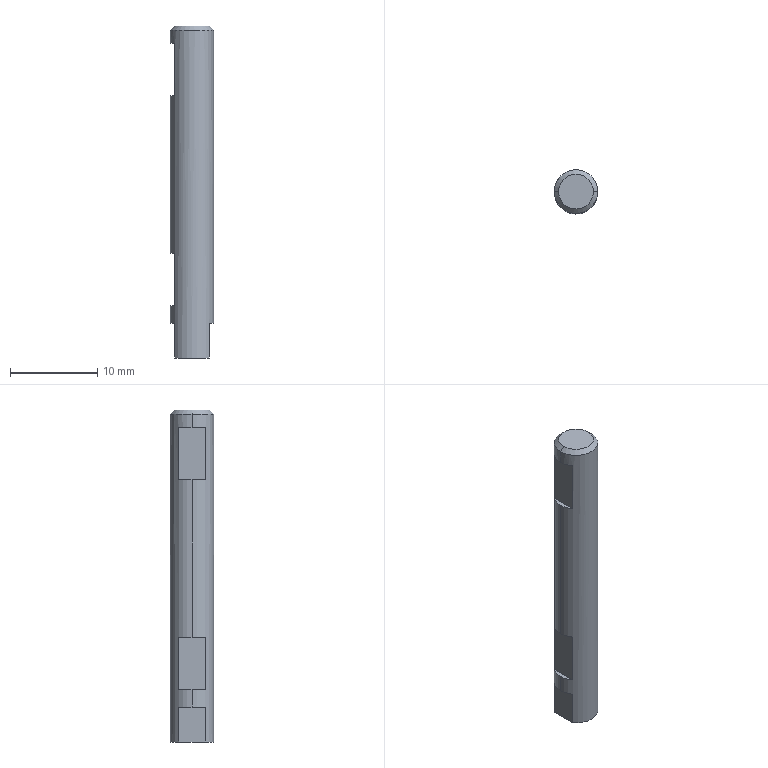Part | STEP file | PN_0012 Mount electronic clip wheel shaft A | 1 solid | 16 faces | box 5 x 5 x 38 mm | volume 723.858 mm3 | plane 12 | cone 2 | cylinder 2 | commonest cylinder face diameters 5 x2
STEP:
#1=CARTESIAN_POINT('',(0.,0.,0.));
#2=DIRECTION('',(0.,0.,1.));
#3=DIRECTION('',(1.,0.,0.));
#4=AXIS2_PLACEMENT_3D('',#1,#2,#3);
#5=CARTESIAN_POINT('',(2.,0.,38.));
#6=VERTEX_POINT('',#5);
#7=CARTESIAN_POINT('',(-2.,0.,38.));
#8=VERTEX_POINT('',#7);
#9=CARTESIAN_POINT('',(0.,0.,38.));
#10=DIRECTION('',(0.,0.,1.));
#11=DIRECTION('',(1.,0.,0.));
#12=AXIS2_PLACEMENT_3D('',#9,#10,#11);
#13=CIRCLE('',#12,2.);
#14=CARTESIAN_POINT('',(0.,0.,38.));
#15=DIRECTION('',(0.,0.,-1.));
#16=DIRECTION('',(-1.,0.,0.));
#17=AXIS2_PLACEMENT_3D('',#14,#15,#16);
#18=CONICAL_SURFACE('',#17,2.,0.7854);
#19=CARTESIAN_POINT('',(3.142,0.));
#20=DIRECTION('',(-1.,0.));
#21=VECTOR('',#20,1.);
#22=LINE('',#19,#21);
#23=(GEOMETRIC_REPRESENTATION_CONTEXT(2)PARAMETRIC_REPRESENTATION_CONTEXT()REPRESENTATION_CONTEXT('',''));
#24=DEFINITIONAL_REPRESENTATION('',(#22),#23);
#25=PCURVE('',#18,#24);
#26=CARTESIAN_POINT('',(0.,0.,38.));
#27=DIRECTION('',(0.,0.,1.));
#28=DIRECTION('',(1.,0.,0.));
#29=AXIS2_PLACEMENT_3D('',#26,#27,#28);
#30=PLANE('',#29);
#31=CARTESIAN_POINT('',(0.,0.));
#32=DIRECTION('',(1.,0.));
#33=AXIS2_PLACEMENT_2D('',#31,#32);
#34=CIRCLE('',#33,2.);
#35=(GEOMETRIC_REPRESENTATION_CONTEXT(2)PARAMETRIC_REPRESENTATION_CONTEXT()REPRESENTATION_CONTEXT('',''));
#36=DEFINITIONAL_REPRESENTATION('',(#34),#35);
#37=PCURVE('',#30,#36);
#38=SURFACE_CURVE('',#13,(#25,#37),.PCURVE_S1.);
#39=EDGE_CURVE('',#6,#8,#38,.T.);
#40=ORIENTED_EDGE('',*,*,#39,.F.);
#41=CARTESIAN_POINT('',(2.5,0.,37.5));
#42=VERTEX_POINT('',#41);
#43=CARTESIAN_POINT('',(2.,0.,38.));
#44=DIRECTION('',(0.7071,0.,-0.7071));
#45=VECTOR('',#44,1.);
#46=LINE('',#43,#45);
#47=CARTESIAN_POINT('',(3.142,0.));
#48=DIRECTION('',(0.,1.));
#49=VECTOR('',#48,1.);
#50=LINE('',#47,#49);
#51=(GEOMETRIC_REPRESENTATION_CONTEXT(2)PARAMETRIC_REPRESENTATION_CONTEXT()REPRESENTATION_CONTEXT('',''));
#52=DEFINITIONAL_REPRESENTATION('',(#50),#51);
#53=PCURVE('',#18,#52);
#54=CARTESIAN_POINT('',(0.,0.,38.));
#55=DIRECTION('',(0.,0.,-1.));
#56=DIRECTION('',(-1.,0.,0.));
#57=AXIS2_PLACEMENT_3D('',#54,#55,#56);
#58=CONICAL_SURFACE('',#57,2.,0.7854);
#59=CARTESIAN_POINT('',(3.142,0.));
#60=DIRECTION('',(0.,1.));
#61=VECTOR('',#60,1.);
#62=LINE('',#59,#61);
#63=(GEOMETRIC_REPRESENTATION_CONTEXT(2)PARAMETRIC_REPRESENTATION_CONTEXT()REPRESENTATION_CONTEXT('',''));
#64=DEFINITIONAL_REPRESENTATION('',(#62),#63);
#65=PCURVE('',#58,#64);
#66=SURFACE_CURVE('',#46,(#53,#65),.PCURVE_S1.);
#67=EDGE_CURVE('',#6,#42,#66,.T.);
#68=ORIENTED_EDGE('',*,*,#67,.T.);
#69=CARTESIAN_POINT('',(-2.5,0.,37.5));
#70=VERTEX_POINT('',#69);
#71=CARTESIAN_POINT('',(0.,0.,37.5));
#72=DIRECTION('',(0.,0.,-1.));
#73=DIRECTION('',(1.,0.,0.));
#74=AXIS2_PLACEMENT_3D('',#71,#72,#73);
#75=CIRCLE('',#74,2.5);
#76=CARTESIAN_POINT('',(-3.142,0.5));
#77=DIRECTION('',(1.,0.));
#78=VECTOR('',#77,1.);
#79=LINE('',#76,#78);
#80=(GEOMETRIC_REPRESENTATION_CONTEXT(2)PARAMETRIC_REPRESENTATION_CONTEXT()REPRESENTATION_CONTEXT('',''));
#81=DEFINITIONAL_REPRESENTATION('',(#79),#80);
#82=PCURVE('',#18,#81);
#83=CARTESIAN_POINT('',(0.,0.,38.));
#84=DIRECTION('',(0.,0.,-1.));
#85=DIRECTION('',(-1.,0.,0.));
#86=AXIS2_PLACEMENT_3D('',#83,#84,#85);
#87=CYLINDRICAL_SURFACE('',#86,2.5);
#88=CARTESIAN_POINT('',(-3.142,0.5));
#89=DIRECTION('',(1.,0.));
#90=VECTOR('',#89,1.);
#91=LINE('',#88,#90);
#92=(GEOMETRIC_REPRESENTATION_CONTEXT(2)PARAMETRIC_REPRESENTATION_CONTEXT()REPRESENTATION_CONTEXT('',''));
#93=DEFINITIONAL_REPRESENTATION('',(#91),#92);
#94=PCURVE('',#87,#93);
#95=SURFACE_CURVE('',#75,(#82,#94),.PCURVE_S1.);
#96=EDGE_CURVE('',#70,#42,#95,.T.);
#97=ORIENTED_EDGE('',*,*,#96,.F.);
#98=CARTESIAN_POINT('',(-2.,0.,38.));
#99=DIRECTION('',(-0.7071,0.,-0.7071));
#100=VECTOR('',#99,1.);
#101=LINE('',#98,#100);
#102=CARTESIAN_POINT('',(0.,0.));
#103=DIRECTION('',(0.,1.));
#104=VECTOR('',#103,1.);
#105=LINE('',#102,#104);
#106=(GEOMETRIC_REPRESENTATION_CONTEXT(2)PARAMETRIC_REPRESENTATION_CONTEXT()REPRESENTATION_CONTEXT('',''));
#107=DEFINITIONAL_REPRESENTATION('',(#105),#106);
#108=PCURVE('',#18,#107);
#109=CARTESIAN_POINT('',(6.283,0.));
#110=DIRECTION('',(0.,1.));
#111=VECTOR('',#110,1.);
#112=LINE('',#109,#111);
#113=(GEOMETRIC_REPRESENTATION_CONTEXT(2)PARAMETRIC_REPRESENTATION_CONTEXT()REPRESENTATION_CONTEXT('',''));
#114=DEFINITIONAL_REPRESENTATION('',(#112),#113);
#115=PCURVE('',#58,#114);
#116=SURFACE_CURVE('',#101,(#108,#115),.PCURVE_S1.);
#117=EDGE_CURVE('',#8,#70,#116,.T.);
#118=ORIENTED_EDGE('',*,*,#117,.F.);
#119=EDGE_LOOP('',(#40,#68,#97,#118));
#120=FACE_BOUND('',#119,.T.);
#121=ADVANCED_FACE('',(#120),#18,.T.);
#122=ORIENTED_EDGE('',*,*,#96,.T.);
#123=CARTESIAN_POINT('',(2.5,0.,4.));
#124=VERTEX_POINT('',#123);
#125=CARTESIAN_POINT('',(2.5,0.,38.));
#126=DIRECTION('',(0.,0.,-1.));
#127=VECTOR('',#126,1.);
#128=LINE('',#125,#127);
#129=CARTESIAN_POINT('',(3.142,0.));
#130=DIRECTION('',(0.,1.));
#131=VECTOR('',#130,1.);
#132=LINE('',#129,#131);
#133=(GEOMETRIC_REPRESENTATION_CONTEXT(2)PARAMETRIC_REPRESENTATION_CONTEXT()REPRESENTATION_CONTEXT('',''));
#134=DEFINITIONAL_REPRESENTATION('',(#132),#133);
#135=PCURVE('',#87,#134);
#136=CARTESIAN_POINT('',(0.,0.,38.));
#137=DIRECTION('',(0.,0.,-1.));
#138=DIRECTION('',(-1.,0.,0.));
#139=AXIS2_PLACEMENT_3D('',#136,#137,#138);
#140=CYLINDRICAL_SURFACE('',#139,2.5);
#141=CARTESIAN_POINT('',(3.142,0.));
#142=DIRECTION('',(0.,1.));
#143=VECTOR('',#142,1.);
#144=LINE('',#141,#143);
#145=(GEOMETRIC_REPRESENTATION_CONTEXT(2)PARAMETRIC_REPRESENTATION_CONTEXT()REPRESENTATION_CONTEXT('',''));
#146=DEFINITIONAL_REPRESENTATION('',(#144),#145);
#147=PCURVE('',#140,#146);
#148=SURFACE_CURVE('',#128,(#135,#147),.PCURVE_S1.);
#149=EDGE_CURVE('',#42,#124,#148,.T.);
#150=ORIENTED_EDGE('',*,*,#149,.T.);
#151=CARTESIAN_POINT('',(2.,1.5,4.));
#152=VERTEX_POINT('',#151);
#153=CARTESIAN_POINT('',(0.,0.,4.));
#154=DIRECTION('',(0.,0.,-1.));
#155=DIRECTION('',(-1.,0.,0.));
#156=AXIS2_PLACEMENT_3D('',#153,#154,#155);
#157=CIRCLE('',#156,2.5);
#158=CARTESIAN_POINT('',(0.,34.));
#159=DIRECTION('',(1.,0.));
#160=VECTOR('',#159,1.);
#161=LINE('',#158,#160);
#162=(GEOMETRIC_REPRESENTATION_CONTEXT(2)PARAMETRIC_REPRESENTATION_CONTEXT()REPRESENTATION_CONTEXT('',''));
#163=DEFINITIONAL_REPRESENTATION('',(#161),#162);
#164=PCURVE('',#87,#163);
#165=CARTESIAN_POINT('',(0.,0.,4.));
#166=DIRECTION('',(0.,0.,-1.));
#167=DIRECTION('',(-1.,0.,0.));
#168=AXIS2_PLACEMENT_3D('',#165,#166,#167);
#169=PLANE('',#168);
#170=CARTESIAN_POINT('',(0.,0.));
#171=DIRECTION('',(1.,0.));
#172=AXIS2_PLACEMENT_2D('',#170,#171);
#173=CIRCLE('',#172,2.5);
#174=(GEOMETRIC_REPRESENTATION_CONTEXT(2)PARAMETRIC_REPRESENTATION_CONTEXT()REPRESENTATION_CONTEXT('',''));
#175=DEFINITIONAL_REPRESENTATION('',(#173),#174);
#176=PCURVE('',#169,#175);
#177=SURFACE_CURVE('',#157,(#164,#176),.PCURVE_S1.);
#178=EDGE_CURVE('',#152,#124,#177,.T.);
#179=ORIENTED_EDGE('',*,*,#178,.F.);
#180=CARTESIAN_POINT('',(2.,1.5,0.));
#181=VERTEX_POINT('',#180);
#182=CARTESIAN_POINT('',(2.,1.5,38.));
#183=DIRECTION('',(0.,0.,-1.));
#184=VECTOR('',#183,1.);
#185=LINE('',#182,#184);
#186=CARTESIAN_POINT('',(2.498,0.));
#187=DIRECTION('',(0.,1.));
#188=VECTOR('',#187,1.);
#189=LINE('',#186,#188);
#190=(GEOMETRIC_REPRESENTATION_CONTEXT(2)PARAMETRIC_REPRESENTATION_CONTEXT()REPRESENTATION_CONTEXT('',''));
#191=DEFINITIONAL_REPRESENTATION('',(#189),#190);
#192=PCURVE('',#87,#191);
#193=CARTESIAN_POINT('',(2.,0.,4.));
#194=DIRECTION('',(-1.,0.,0.));
#195=DIRECTION('',(0.,0.,1.));
#196=AXIS2_PLACEMENT_3D('',#193,#194,#195);
#197=PLANE('',#196);
#198=CARTESIAN_POINT('',(34.,1.5));
#199=DIRECTION('',(-1.,0.));
#200=VECTOR('',#199,1.);
#201=LINE('',#198,#200);
#202=(GEOMETRIC_REPRESENTATION_CONTEXT(2)PARAMETRIC_REPRESENTATION_CONTEXT()REPRESENTATION_CONTEXT('',''));
#203=DEFINITIONAL_REPRESENTATION('',(#201),#202);
#204=PCURVE('',#197,#203);
#205=SURFACE_CURVE('',#185,(#192,#204),.PCURVE_S1.);
#206=EDGE_CURVE('',#152,#181,#205,.T.);
#207=ORIENTED_EDGE('',*,*,#206,.T.);
#208=CARTESIAN_POINT('',(-2.,1.5,0.));
#209=VERTEX_POINT('',#208);
#210=CARTESIAN_POINT('',(0.,0.,0.));
#211=DIRECTION('',(0.,0.,1.));
#212=DIRECTION('',(1.,0.,0.));
#213=AXIS2_PLACEMENT_3D('',#210,#211,#212);
#214=CIRCLE('',#213,2.5);
#215=CARTESIAN_POINT('',(3.142,38.));
#216=DIRECTION('',(-1.,0.));
#217=VECTOR('',#216,1.);
#218=LINE('',#215,#217);
#219=(GEOMETRIC_REPRESENTATION_CONTEXT(2)PARAMETRIC_REPRESENTATION_CONTEXT()REPRESENTATION_CONTEXT('',''));
#220=DEFINITIONAL_REPRESENTATION('',(#218),#219);
#221=PCURVE('',#87,#220);
#222=CARTESIAN_POINT('',(0.,0.,0.));
#223=DIRECTION('',(0.,0.,1.));
#224=DIRECTION('',(1.,0.,0.));
#225=AXIS2_PLACEMENT_3D('',#222,#223,#224);
#226=PLANE('',#225);
#227=CARTESIAN_POINT('',(0.,0.));
#228=DIRECTION('',(1.,0.));
#229=AXIS2_PLACEMENT_2D('',#227,#228);
#230=CIRCLE('',#229,2.5);
#231=(GEOMETRIC_REPRESENTATION_CONTEXT(2)PARAMETRIC_REPRESENTATION_CONTEXT()REPRESENTATION_CONTEXT('',''));
#232=DEFINITIONAL_REPRESENTATION('',(#230),#231);
#233=PCURVE('',#226,#232);
#234=SURFACE_CURVE('',#214,(#221,#233),.PCURVE_S1.);
#235=EDGE_CURVE('',#181,#209,#234,.T.);
#236=ORIENTED_EDGE('',*,*,#235,.T.);
#237=CARTESIAN_POINT('',(-2.,1.5,4.));
#238=VERTEX_POINT('',#237);
#239=CARTESIAN_POINT('',(-2.,1.5,38.));
#240=DIRECTION('',(0.,0.,-1.));
#241=VECTOR('',#240,1.);
#242=LINE('',#239,#241);
#243=CARTESIAN_POINT('',(0.6435,0.));
#244=DIRECTION('',(0.,1.));
#245=VECTOR('',#244,1.);
#246=LINE('',#243,#245);
#247=(GEOMETRIC_REPRESENTATION_CONTEXT(2)PARAMETRIC_REPRESENTATION_CONTEXT()REPRESENTATION_CONTEXT('',''));
#248=DEFINITIONAL_REPRESENTATION('',(#246),#247);
#249=PCURVE('',#87,#248);
#250=CARTESIAN_POINT('',(-2.,0.,4.));
#251=DIRECTION('',(-1.,0.,0.));
#252=DIRECTION('',(0.,0.,1.));
#253=AXIS2_PLACEMENT_3D('',#250,#251,#252);
#254=PLANE('',#253);
#255=CARTESIAN_POINT('',(34.,1.5));
#256=DIRECTION('',(-1.,0.));
#257=VECTOR('',#256,1.);
#258=LINE('',#255,#257);
#259=(GEOMETRIC_REPRESENTATION_CONTEXT(2)PARAMETRIC_REPRESENTATION_CONTEXT()REPRESENTATION_CONTEXT('',''));
#260=DEFINITIONAL_REPRESENTATION('',(#258),#259);
#261=PCURVE('',#254,#260);
#262=SURFACE_CURVE('',#242,(#249,#261),.PCURVE_S1.);
#263=EDGE_CURVE('',#238,#209,#262,.T.);
#264=ORIENTED_EDGE('',*,*,#263,.F.);
#265=CARTESIAN_POINT('',(-2.5,0.,4.));
#266=VERTEX_POINT('',#265);
#267=CARTESIAN_POINT('',(0.,0.,4.));
#268=DIRECTION('',(0.,0.,-1.));
#269=DIRECTION('',(-1.,0.,0.));
#270=AXIS2_PLACEMENT_3D('',#267,#268,#269);
#271=CIRCLE('',#270,2.5);
#272=CARTESIAN_POINT('',(0.,34.));
#273=DIRECTION('',(1.,0.));
#274=VECTOR('',#273,1.);
#275=LINE('',#272,#274);
#276=(GEOMETRIC_REPRESENTATION_CONTEXT(2)PARAMETRIC_REPRESENTATION_CONTEXT()REPRESENTATION_CONTEXT('',''));
#277=DEFINITIONAL_REPRESENTATION('',(#275),#276);
#278=PCURVE('',#87,#277);
#279=CARTESIAN_POINT('',(0.,0.,4.));
#280=DIRECTION('',(0.,0.,-1.));
#281=DIRECTION('',(-1.,0.,0.));
#282=AXIS2_PLACEMENT_3D('',#279,#280,#281);
#283=PLANE('',#282);
#284=CARTESIAN_POINT('',(0.,0.));
#285=DIRECTION('',(1.,0.));
#286=AXIS2_PLACEMENT_2D('',#284,#285);
#287=CIRCLE('',#286,2.5);
#288=(GEOMETRIC_REPRESENTATION_CONTEXT(2)PARAMETRIC_REPRESENTATION_CONTEXT()REPRESENTATION_CONTEXT('',''));
#289=DEFINITIONAL_REPRESENTATION('',(#287),#288);
#290=PCURVE('',#283,#289);
#291=SURFACE_CURVE('',#271,(#278,#290),.PCURVE_S1.);
#292=EDGE_CURVE('',#266,#238,#291,.T.);
#293=ORIENTED_EDGE('',*,*,#292,.F.);
#294=CARTESIAN_POINT('',(-2.5,0.,6.));
#295=VERTEX_POINT('',#294);
#296=CARTESIAN_POINT('',(-2.5,0.,38.));
#297=DIRECTION('',(0.,0.,-1.));
#298=VECTOR('',#297,1.);
#299=LINE('',#296,#298);
#300=CARTESIAN_POINT('',(0.,0.));
#301=DIRECTION('',(0.,1.));
#302=VECTOR('',#301,1.);
#303=LINE('',#300,#302);
#304=(GEOMETRIC_REPRESENTATION_CONTEXT(2)PARAMETRIC_REPRESENTATION_CONTEXT()REPRESENTATION_CONTEXT('',''));
#305=DEFINITIONAL_REPRESENTATION('',(#303),#304);
#306=PCURVE('',#87,#305);
#307=CARTESIAN_POINT('',(6.283,0.));
#308=DIRECTION('',(0.,1.));
#309=VECTOR('',#308,1.);
#310=LINE('',#307,#309);
#311=(GEOMETRIC_REPRESENTATION_CONTEXT(2)PARAMETRIC_REPRESENTATION_CONTEXT()REPRESENTATION_CONTEXT('',''));
#312=DEFINITIONAL_REPRESENTATION('',(#310),#311);
#313=PCURVE('',#140,#312);
#314=SURFACE_CURVE('',#299,(#306,#313),.PCURVE_S1.);
#315=EDGE_CURVE('',#295,#266,#314,.T.);
#316=ORIENTED_EDGE('',*,*,#315,.F.);
#317=CARTESIAN_POINT('',(-2.,1.5,6.));
#318=VERTEX_POINT('',#317);
#319=CARTESIAN_POINT('',(0.,0.,6.));
#320=DIRECTION('',(0.,0.,1.));
#321=DIRECTION('',(1.,0.,0.));
#322=AXIS2_PLACEMENT_3D('',#319,#320,#321);
#323=CIRCLE('',#322,2.5);
#324=CARTESIAN_POINT('',(3.142,32.));
#325=DIRECTION('',(-1.,0.));
#326=VECTOR('',#325,1.);
#327=LINE('',#324,#326);
#328=(GEOMETRIC_REPRESENTATION_CONTEXT(2)PARAMETRIC_REPRESENTATION_CONTEXT()REPRESENTATION_CONTEXT('',''));
#329=DEFINITIONAL_REPRESENTATION('',(#327),#328);
#330=PCURVE('',#87,#329);
#331=CARTESIAN_POINT('',(-5.963,40.,6.));
#332=DIRECTION('',(0.,0.,1.));
#333=DIRECTION('',(1.,0.,0.));
#334=AXIS2_PLACEMENT_3D('',#331,#332,#333);
#335=PLANE('',#334);
#336=CARTESIAN_POINT('',(5.963,-40.));
#337=DIRECTION('',(1.,0.));
#338=AXIS2_PLACEMENT_2D('',#336,#337);
#339=CIRCLE('',#338,2.5);
#340=(GEOMETRIC_REPRESENTATION_CONTEXT(2)PARAMETRIC_REPRESENTATION_CONTEXT()REPRESENTATION_CONTEXT('',''));
#341=DEFINITIONAL_REPRESENTATION('',(#339),#340);
#342=PCURVE('',#335,#341);
#343=SURFACE_CURVE('',#323,(#330,#342),.PCURVE_S1.);
#344=EDGE_CURVE('',#318,#295,#343,.T.);
#345=ORIENTED_EDGE('',*,*,#344,.F.);
#346=CARTESIAN_POINT('',(-2.,1.5,12.));
#347=VERTEX_POINT('',#346);
#348=CARTESIAN_POINT('',(-2.,1.5,38.));
#349=DIRECTION('',(0.,0.,-1.));
#350=VECTOR('',#349,1.);
#351=LINE('',#348,#350);
#352=CARTESIAN_POINT('',(0.6435,0.));
#353=DIRECTION('',(0.,1.));
#354=VECTOR('',#353,1.);
#355=LINE('',#352,#354);
#356=(GEOMETRIC_REPRESENTATION_CONTEXT(2)PARAMETRIC_REPRESENTATION_CONTEXT()REPRESENTATION_CONTEXT('',''));
#357=DEFINITIONAL_REPRESENTATION('',(#355),#356);
#358=PCURVE('',#87,#357);
#359=CARTESIAN_POINT('',(-2.,40.,6.));
#360=DIRECTION('',(-1.,0.,0.));
#361=DIRECTION('',(0.,0.,1.));
#362=AXIS2_PLACEMENT_3D('',#359,#360,#361);
#363=PLANE('',#362);
#364=CARTESIAN_POINT('',(32.,-38.5));
#365=DIRECTION('',(-1.,0.));
#366=VECTOR('',#365,1.);
#367=LINE('',#364,#366);
#368=(GEOMETRIC_REPRESENTATION_CONTEXT(2)PARAMETRIC_REPRESENTATION_CONTEXT()REPRESENTATION_CONTEXT('',''));
#369=DEFINITIONAL_REPRESENTATION('',(#367),#368);
#370=PCURVE('',#363,#369);
#371=SURFACE_CURVE('',#351,(#358,#370),.PCURVE_S1.);
#372=EDGE_CURVE('',#347,#318,#371,.T.);
#373=ORIENTED_EDGE('',*,*,#372,.F.);
#374=CARTESIAN_POINT('',(-2.5,0.,12.));
#375=VERTEX_POINT('',#374);
#376=CARTESIAN_POINT('',(0.,0.,12.));
#377=DIRECTION('',(0.,0.,-1.));
#378=DIRECTION('',(-1.,0.,0.));
#379=AXIS2_PLACEMENT_3D('',#376,#377,#378);
#380=CIRCLE('',#379,2.5);
#381=CARTESIAN_POINT('',(0.,26.));
#382=DIRECTION('',(1.,0.));
#383=VECTOR('',#382,1.);
#384=LINE('',#381,#383);
#385=(GEOMETRIC_REPRESENTATION_CONTEXT(2)PARAMETRIC_REPRESENTATION_CONTEXT()REPRESENTATION_CONTEXT('',''));
#386=DEFINITIONAL_REPRESENTATION('',(#384),#385);
#387=PCURVE('',#87,#386);
#388=CARTESIAN_POINT('',(-5.963,40.,12.));
#389=DIRECTION('',(0.,0.,-1.));
#390=DIRECTION('',(-1.,0.,0.));
#391=AXIS2_PLACEMENT_3D('',#388,#389,#390);
#392=PLANE('',#391);
#393=CARTESIAN_POINT('',(-5.963,-40.));
#394=DIRECTION('',(1.,0.));
#395=AXIS2_PLACEMENT_2D('',#393,#394);
#396=CIRCLE('',#395,2.5);
#397=(GEOMETRIC_REPRESENTATION_CONTEXT(2)PARAMETRIC_REPRESENTATION_CONTEXT()REPRESENTATION_CONTEXT('',''));
#398=DEFINITIONAL_REPRESENTATION('',(#396),#397);
#399=PCURVE('',#392,#398);
#400=SURFACE_CURVE('',#380,(#387,#399),.PCURVE_S1.);
#401=EDGE_CURVE('',#375,#347,#400,.T.);
#402=ORIENTED_EDGE('',*,*,#401,.F.);
#403=CARTESIAN_POINT('',(-2.5,0.,30.));
#404=VERTEX_POINT('',#403);
#405=CARTESIAN_POINT('',(-2.5,0.,38.));
#406=DIRECTION('',(0.,0.,-1.));
#407=VECTOR('',#406,1.);
#408=LINE('',#405,#407);
#409=CARTESIAN_POINT('',(0.,0.));
#410=DIRECTION('',(0.,1.));
#411=VECTOR('',#410,1.);
#412=LINE('',#409,#411);
#413=(GEOMETRIC_REPRESENTATION_CONTEXT(2)PARAMETRIC_REPRESENTATION_CONTEXT()REPRESENTATION_CONTEXT('',''));
#414=DEFINITIONAL_REPRESENTATION('',(#412),#413);
#415=PCURVE('',#87,#414);
#416=CARTESIAN_POINT('',(6.283,0.));
#417=DIRECTION('',(0.,1.));
#418=VECTOR('',#417,1.);
#419=LINE('',#416,#418);
#420=(GEOMETRIC_REPRESENTATION_CONTEXT(2)PARAMETRIC_REPRESENTATION_CONTEXT()REPRESENTATION_CONTEXT('',''));
#421=DEFINITIONAL_REPRESENTATION('',(#419),#420);
#422=PCURVE('',#140,#421);
#423=SURFACE_CURVE('',#408,(#415,#422),.PCURVE_S1.);
#424=EDGE_CURVE('',#404,#375,#423,.T.);
#425=ORIENTED_EDGE('',*,*,#424,.F.);
#426=CARTESIAN_POINT('',(-2.,1.5,30.));
#427=VERTEX_POINT('',#426);
#428=CARTESIAN_POINT('',(0.,0.,30.));
#429=DIRECTION('',(0.,0.,1.));
#430=DIRECTION('',(1.,0.,0.));
#431=AXIS2_PLACEMENT_3D('',#428,#429,#430);
#432=CIRCLE('',#431,2.5);
#433=CARTESIAN_POINT('',(3.142,8.));
#434=DIRECTION('',(-1.,0.));
#435=VECTOR('',#434,1.);
#436=LINE('',#433,#435);
#437=(GEOMETRIC_REPRESENTATION_CONTEXT(2)PARAMETRIC_REPRESENTATION_CONTEXT()REPRESENTATION_CONTEXT('',''));
#438=DEFINITIONAL_REPRESENTATION('',(#436),#437);
#439=PCURVE('',#87,#438);
#440=CARTESIAN_POINT('',(-4.8,40.,30.));
#441=DIRECTION('',(0.,0.,1.));
#442=DIRECTION('',(1.,0.,0.));
#443=AXIS2_PLACEMENT_3D('',#440,#441,#442);
#444=PLANE('',#443);
#445=CARTESIAN_POINT('',(4.8,-40.));
#446=DIRECTION('',(1.,0.));
#447=AXIS2_PLACEMENT_2D('',#445,#446);
#448=CIRCLE('',#447,2.5);
#449=(GEOMETRIC_REPRESENTATION_CONTEXT(2)PARAMETRIC_REPRESENTATION_CONTEXT()REPRESENTATION_CONTEXT('',''));
#450=DEFINITIONAL_REPRESENTATION('',(#448),#449);
#451=PCURVE('',#444,#450);
#452=SURFACE_CURVE('',#432,(#439,#451),.PCURVE_S1.);
#453=EDGE_CURVE('',#427,#404,#452,.T.);
#454=ORIENTED_EDGE('',*,*,#453,.F.);
#455=CARTESIAN_POINT('',(-2.,1.5,36.));
#456=VERTEX_POINT('',#455);
#457=CARTESIAN_POINT('',(-2.,1.5,38.));
#458=DIRECTION('',(0.,0.,-1.));
#459=VECTOR('',#458,1.);
#460=LINE('',#457,#459);
#461=CARTESIAN_POINT('',(0.6435,0.));
#462=DIRECTION('',(0.,1.));
#463=VECTOR('',#462,1.);
#464=LINE('',#461,#463);
#465=(GEOMETRIC_REPRESENTATION_CONTEXT(2)PARAMETRIC_REPRESENTATION_CONTEXT()REPRESENTATION_CONTEXT('',''));
#466=DEFINITIONAL_REPRESENTATION('',(#464),#465);
#467=PCURVE('',#87,#466);
#468=CARTESIAN_POINT('',(-2.,40.,30.));
#469=DIRECTION('',(-1.,0.,0.));
#470=DIRECTION('',(0.,0.,1.));
#471=AXIS2_PLACEMENT_3D('',#468,#469,#470);
#472=PLANE('',#471);
#473=CARTESIAN_POINT('',(8.,-38.5));
#474=DIRECTION('',(-1.,0.));
#475=VECTOR('',#474,1.);
#476=LINE('',#473,#475);
#477=(GEOMETRIC_REPRESENTATION_CONTEXT(2)PARAMETRIC_REPRESENTATION_CONTEXT()REPRESENTATION_CONTEXT('',''));
#478=DEFINITIONAL_REPRESENTATION('',(#476),#477);
#479=PCURVE('',#472,#478);
#480=SURFACE_CURVE('',#460,(#467,#479),.PCURVE_S1.);
#481=EDGE_CURVE('',#456,#427,#480,.T.);
#482=ORIENTED_EDGE('',*,*,#481,.F.);
#483=CARTESIAN_POINT('',(-2.5,0.,36.));
#484=VERTEX_POINT('',#483);
#485=CARTESIAN_POINT('',(0.,0.,36.));
#486=DIRECTION('',(0.,0.,-1.));
#487=DIRECTION('',(-1.,0.,0.));
#488=AXIS2_PLACEMENT_3D('',#485,#486,#487);
#489=CIRCLE('',#488,2.5);
#490=CARTESIAN_POINT('',(0.,2.));
#491=DIRECTION('',(1.,0.));
#492=VECTOR('',#491,1.);
#493=LINE('',#490,#492);
#494=(GEOMETRIC_REPRESENTATION_CONTEXT(2)PARAMETRIC_REPRESENTATION_CONTEXT()REPRESENTATION_CONTEXT('',''));
#495=DEFINITIONAL_REPRESENTATION('',(#493),#494);
#496=PCURVE('',#87,#495);
#497=CARTESIAN_POINT('',(-4.8,40.,36.));
#498=DIRECTION('',(0.,0.,-1.));
#499=DIRECTION('',(-1.,0.,0.));
#500=AXIS2_PLACEMENT_3D('',#497,#498,#499);
#501=PLANE('',#500);
#502=CARTESIAN_POINT('',(-4.8,-40.));
#503=DIRECTION('',(1.,0.));
#504=AXIS2_PLACEMENT_2D('',#502,#503);
#505=CIRCLE('',#504,2.5);
#506=(GEOMETRIC_REPRESENTATION_CONTEXT(2)PARAMETRIC_REPRESENTATION_CONTEXT()REPRESENTATION_CONTEXT('',''));
#507=DEFINITIONAL_REPRESENTATION('',(#505),#506);
#508=PCURVE('',#501,#507);
#509=SURFACE_CURVE('',#489,(#496,#508),.PCURVE_S1.);
#510=EDGE_CURVE('',#484,#456,#509,.T.);
#511=ORIENTED_EDGE('',*,*,#510,.F.);
#512=CARTESIAN_POINT('',(-2.5,0.,38.));
#513=DIRECTION('',(0.,0.,-1.));
#514=VECTOR('',#513,1.);
#515=LINE('',#512,#514);
#516=CARTESIAN_POINT('',(0.,0.));
#517=DIRECTION('',(0.,1.));
#518=VECTOR('',#517,1.);
#519=LINE('',#516,#518);
#520=(GEOMETRIC_REPRESENTATION_CONTEXT(2)PARAMETRIC_REPRESENTATION_CONTEXT()REPRESENTATION_CONTEXT('',''));
#521=DEFINITIONAL_REPRESENTATION('',(#519),#520);
#522=PCURVE('',#87,#521);
#523=CARTESIAN_POINT('',(6.283,0.));
#524=DIRECTION('',(0.,1.));
#525=VECTOR('',#524,1.);
#526=LINE('',#523,#525);
#527=(GEOMETRIC_REPRESENTATION_CONTEXT(2)PARAMETRIC_REPRESENTATION_CONTEXT()REPRESENTATION_CONTEXT('',''));
#528=DEFINITIONAL_REPRESENTATION('',(#526),#527);
#529=PCURVE('',#140,#528);
#530=SURFACE_CURVE('',#515,(#522,#529),.PCURVE_S1.);
#531=EDGE_CURVE('',#70,#484,#530,.T.);
#532=ORIENTED_EDGE('',*,*,#531,.F.);
#533=EDGE_LOOP('',(#122,#150,#179,#207,#236,#264,#293,#316,#345,#373,#402,#425,#454,#482,#511,#532));
#534=FACE_BOUND('',#533,.T.);
#535=ADVANCED_FACE('',(#534),#87,.T.);
#536=ORIENTED_EDGE('',*,*,#149,.F.);
#537=CARTESIAN_POINT('',(0.,0.,37.5));
#538=DIRECTION('',(0.,0.,-1.));
#539=DIRECTION('',(1.,0.,0.));
#540=AXIS2_PLACEMENT_3D('',#537,#538,#539);
#541=CIRCLE('',#540,2.5);
#542=CARTESIAN_POINT('',(3.142,0.5));
#543=DIRECTION('',(1.,0.));
#544=VECTOR('',#543,1.);
#545=LINE('',#542,#544);
#546=(GEOMETRIC_REPRESENTATION_CONTEXT(2)PARAMETRIC_REPRESENTATION_CONTEXT()REPRESENTATION_CONTEXT('',''));
#547=DEFINITIONAL_REPRESENTATION('',(#545),#546);
#548=PCURVE('',#140,#547);
#549=CARTESIAN_POINT('',(3.142,0.5));
#550=DIRECTION('',(1.,0.));
#551=VECTOR('',#550,1.);
#552=LINE('',#549,#551);
#553=(GEOMETRIC_REPRESENTATION_CONTEXT(2)PARAMETRIC_REPRESENTATION_CONTEXT()REPRESENTATION_CONTEXT('',''));
#554=DEFINITIONAL_REPRESENTATION('',(#552),#553);
#555=PCURVE('',#58,#554);
#556=SURFACE_CURVE('',#541,(#548,#555),.PCURVE_S1.);
#557=EDGE_CURVE('',#42,#70,#556,.T.);
#558=ORIENTED_EDGE('',*,*,#557,.T.);
#559=ORIENTED_EDGE('',*,*,#531,.T.);
#560=CARTESIAN_POINT('',(-2.,-1.5,36.));
#561=VERTEX_POINT('',#560);
#562=CARTESIAN_POINT('',(0.,0.,36.));
#563=DIRECTION('',(0.,0.,-1.));
#564=DIRECTION('',(-1.,0.,0.));
#565=AXIS2_PLACEMENT_3D('',#562,#563,#564);
#566=CIRCLE('',#565,2.5);
#567=CARTESIAN_POINT('',(0.,2.));
#568=DIRECTION('',(1.,0.));
#569=VECTOR('',#568,1.);
#570=LINE('',#567,#569);
#571=(GEOMETRIC_REPRESENTATION_CONTEXT(2)PARAMETRIC_REPRESENTATION_CONTEXT()REPRESENTATION_CONTEXT('',''));
#572=DEFINITIONAL_REPRESENTATION('',(#570),#571);
#573=PCURVE('',#140,#572);
#574=CARTESIAN_POINT('',(-4.8,-40.));
#575=DIRECTION('',(1.,0.));
#576=AXIS2_PLACEMENT_2D('',#574,#575);
#577=CIRCLE('',#576,2.5);
#578=(GEOMETRIC_REPRESENTATION_CONTEXT(2)PARAMETRIC_REPRESENTATION_CONTEXT()REPRESENTATION_CONTEXT('',''));
#579=DEFINITIONAL_REPRESENTATION('',(#577),#578);
#580=PCURVE('',#501,#579);
#581=SURFACE_CURVE('',#566,(#573,#580),.PCURVE_S1.);
#582=EDGE_CURVE('',#561,#484,#581,.T.);
#583=ORIENTED_EDGE('',*,*,#582,.F.);
#584=CARTESIAN_POINT('',(-2.,-1.5,30.));
#585=VERTEX_POINT('',#584);
#586=CARTESIAN_POINT('',(-2.,-1.5,38.));
#587=DIRECTION('',(0.,0.,1.));
#588=VECTOR('',#587,1.);
#589=LINE('',#586,#588);
#590=CARTESIAN_POINT('',(5.64,0.));
#591=DIRECTION('',(0.,-1.));
#592=VECTOR('',#591,1.);
#593=LINE('',#590,#592);
#594=(GEOMETRIC_REPRESENTATION_CONTEXT(2)PARAMETRIC_REPRESENTATION_CONTEXT()REPRESENTATION_CONTEXT('',''));
#595=DEFINITIONAL_REPRESENTATION('',(#593),#594);
#596=PCURVE('',#140,#595);
#597=CARTESIAN_POINT('',(8.,-41.5));
#598=DIRECTION('',(1.,0.));
#599=VECTOR('',#598,1.);
#600=LINE('',#597,#599);
#601=(GEOMETRIC_REPRESENTATION_CONTEXT(2)PARAMETRIC_REPRESENTATION_CONTEXT()REPRESENTATION_CONTEXT('',''));
#602=DEFINITIONAL_REPRESENTATION('',(#600),#601);
#603=PCURVE('',#472,#602);
#604=SURFACE_CURVE('',#589,(#596,#603),.PCURVE_S1.);
#605=EDGE_CURVE('',#585,#561,#604,.T.);
#606=ORIENTED_EDGE('',*,*,#605,.F.);
#607=CARTESIAN_POINT('',(0.,0.,30.));
#608=DIRECTION('',(0.,0.,1.));
#609=DIRECTION('',(1.,0.,0.));
#610=AXIS2_PLACEMENT_3D('',#607,#608,#609);
#611=CIRCLE('',#610,2.5);
#612=CARTESIAN_POINT('',(9.425,8.));
#613=DIRECTION('',(-1.,0.));
#614=VECTOR('',#613,1.);
#615=LINE('',#612,#614);
#616=(GEOMETRIC_REPRESENTATION_CONTEXT(2)PARAMETRIC_REPRESENTATION_CONTEXT()REPRESENTATION_CONTEXT('',''));
#617=DEFINITIONAL_REPRESENTATION('',(#615),#616);
#618=PCURVE('',#140,#617);
#619=CARTESIAN_POINT('',(4.8,-40.));
#620=DIRECTION('',(1.,0.));
#621=AXIS2_PLACEMENT_2D('',#619,#620);
#622=CIRCLE('',#621,2.5);
#623=(GEOMETRIC_REPRESENTATION_CONTEXT(2)PARAMETRIC_REPRESENTATION_CONTEXT()REPRESENTATION_CONTEXT('',''));
#624=DEFINITIONAL_REPRESENTATION('',(#622),#623);
#625=PCURVE('',#444,#624);
#626=SURFACE_CURVE('',#611,(#618,#625),.PCURVE_S1.);
#627=EDGE_CURVE('',#404,#585,#626,.T.);
#628=ORIENTED_EDGE('',*,*,#627,.F.);
#629=ORIENTED_EDGE('',*,*,#424,.T.);
#630=CARTESIAN_POINT('',(-2.,-1.5,12.));
#631=VERTEX_POINT('',#630);
#632=CARTESIAN_POINT('',(0.,0.,12.));
#633=DIRECTION('',(0.,0.,-1.));
#634=DIRECTION('',(-1.,0.,0.));
#635=AXIS2_PLACEMENT_3D('',#632,#633,#634);
#636=CIRCLE('',#635,2.5);
#637=CARTESIAN_POINT('',(0.,26.));
#638=DIRECTION('',(1.,0.));
#639=VECTOR('',#638,1.);
#640=LINE('',#637,#639);
#641=(GEOMETRIC_REPRESENTATION_CONTEXT(2)PARAMETRIC_REPRESENTATION_CONTEXT()REPRESENTATION_CONTEXT('',''));
#642=DEFINITIONAL_REPRESENTATION('',(#640),#641);
#643=PCURVE('',#140,#642);
#644=CARTESIAN_POINT('',(-5.963,-40.));
#645=DIRECTION('',(1.,0.));
#646=AXIS2_PLACEMENT_2D('',#644,#645);
#647=CIRCLE('',#646,2.5);
#648=(GEOMETRIC_REPRESENTATION_CONTEXT(2)PARAMETRIC_REPRESENTATION_CONTEXT()REPRESENTATION_CONTEXT('',''));
#649=DEFINITIONAL_REPRESENTATION('',(#647),#648);
#650=PCURVE('',#392,#649);
#651=SURFACE_CURVE('',#636,(#643,#650),.PCURVE_S1.);
#652=EDGE_CURVE('',#631,#375,#651,.T.);
#653=ORIENTED_EDGE('',*,*,#652,.F.);
#654=CARTESIAN_POINT('',(-2.,-1.5,6.));
#655=VERTEX_POINT('',#654);
#656=CARTESIAN_POINT('',(-2.,-1.5,38.));
#657=DIRECTION('',(0.,0.,1.));
#658=VECTOR('',#657,1.);
#659=LINE('',#656,#658);
#660=CARTESIAN_POINT('',(5.64,0.));
#661=DIRECTION('',(0.,-1.));
#662=VECTOR('',#661,1.);
#663=LINE('',#660,#662);
#664=(GEOMETRIC_REPRESENTATION_CONTEXT(2)PARAMETRIC_REPRESENTATION_CONTEXT()REPRESENTATION_CONTEXT('',''));
#665=DEFINITIONAL_REPRESENTATION('',(#663),#664);
#666=PCURVE('',#140,#665);
#667=CARTESIAN_POINT('',(32.,-41.5));
#668=DIRECTION('',(1.,0.));
#669=VECTOR('',#668,1.);
#670=LINE('',#667,#669);
#671=(GEOMETRIC_REPRESENTATION_CONTEXT(2)PARAMETRIC_REPRESENTATION_CONTEXT()REPRESENTATION_CONTEXT('',''));
#672=DEFINITIONAL_REPRESENTATION('',(#670),#671);
#673=PCURVE('',#363,#672);
#674=SURFACE_CURVE('',#659,(#666,#673),.PCURVE_S1.);
#675=EDGE_CURVE('',#655,#631,#674,.T.);
#676=ORIENTED_EDGE('',*,*,#675,.F.);
#677=CARTESIAN_POINT('',(0.,0.,6.));
#678=DIRECTION('',(0.,0.,1.));
#679=DIRECTION('',(1.,0.,0.));
#680=AXIS2_PLACEMENT_3D('',#677,#678,#679);
#681=CIRCLE('',#680,2.5);
#682=CARTESIAN_POINT('',(9.425,32.));
#683=DIRECTION('',(-1.,0.));
#684=VECTOR('',#683,1.);
#685=LINE('',#682,#684);
#686=(GEOMETRIC_REPRESENTATION_CONTEXT(2)PARAMETRIC_REPRESENTATION_CONTEXT()REPRESENTATION_CONTEXT('',''));
#687=DEFINITIONAL_REPRESENTATION('',(#685),#686);
#688=PCURVE('',#140,#687);
#689=CARTESIAN_POINT('',(5.963,-40.));
#690=DIRECTION('',(1.,0.));
#691=AXIS2_PLACEMENT_2D('',#689,#690);
#692=CIRCLE('',#691,2.5);
#693=(GEOMETRIC_REPRESENTATION_CONTEXT(2)PARAMETRIC_REPRESENTATION_CONTEXT()REPRESENTATION_CONTEXT('',''));
#694=DEFINITIONAL_REPRESENTATION('',(#692),#693);
#695=PCURVE('',#335,#694);
#696=SURFACE_CURVE('',#681,(#688,#695),.PCURVE_S1.);
#697=EDGE_CURVE('',#295,#655,#696,.T.);
#698=ORIENTED_EDGE('',*,*,#697,.F.);
#699=ORIENTED_EDGE('',*,*,#315,.T.);
#700=CARTESIAN_POINT('',(-2.,-1.5,4.));
#701=VERTEX_POINT('',#700);
#702=CARTESIAN_POINT('',(0.,0.,4.));
#703=DIRECTION('',(0.,0.,-1.));
#704=DIRECTION('',(-1.,0.,0.));
#705=AXIS2_PLACEMENT_3D('',#702,#703,#704);
#706=CIRCLE('',#705,2.5);
#707=CARTESIAN_POINT('',(0.,34.));
#708=DIRECTION('',(1.,0.));
#709=VECTOR('',#708,1.);
#710=LINE('',#707,#709);
#711=(GEOMETRIC_REPRESENTATION_CONTEXT(2)PARAMETRIC_REPRESENTATION_CONTEXT()REPRESENTATION_CONTEXT('',''));
#712=DEFINITIONAL_REPRESENTATION('',(#710),#711);
#713=PCURVE('',#140,#712);
#714=CARTESIAN_POINT('',(0.,0.));
#715=DIRECTION('',(1.,0.));
#716=AXIS2_PLACEMENT_2D('',#714,#715);
#717=CIRCLE('',#716,2.5);
#718=(GEOMETRIC_REPRESENTATION_CONTEXT(2)PARAMETRIC_REPRESENTATION_CONTEXT()REPRESENTATION_CONTEXT('',''));
#719=DEFINITIONAL_REPRESENTATION('',(#717),#718);
#720=PCURVE('',#283,#719);
#721=SURFACE_CURVE('',#706,(#713,#720),.PCURVE_S1.);
#722=EDGE_CURVE('',#701,#266,#721,.T.);
#723=ORIENTED_EDGE('',*,*,#722,.F.);
#724=CARTESIAN_POINT('',(-2.,-1.5,0.));
#725=VERTEX_POINT('',#724);
#726=CARTESIAN_POINT('',(-2.,-1.5,38.));
#727=DIRECTION('',(0.,0.,1.));
#728=VECTOR('',#727,1.);
#729=LINE('',#726,#728);
#730=CARTESIAN_POINT('',(5.64,0.));
#731=DIRECTION('',(0.,-1.));
#732=VECTOR('',#731,1.);
#733=LINE('',#730,#732);
#734=(GEOMETRIC_REPRESENTATION_CONTEXT(2)PARAMETRIC_REPRESENTATION_CONTEXT()REPRESENTATION_CONTEXT('',''));
#735=DEFINITIONAL_REPRESENTATION('',(#733),#734);
#736=PCURVE('',#140,#735);
#737=CARTESIAN_POINT('',(34.,-1.5));
#738=DIRECTION('',(1.,0.));
#739=VECTOR('',#738,1.);
#740=LINE('',#737,#739);
#741=(GEOMETRIC_REPRESENTATION_CONTEXT(2)PARAMETRIC_REPRESENTATION_CONTEXT()REPRESENTATION_CONTEXT('',''));
#742=DEFINITIONAL_REPRESENTATION('',(#740),#741);
#743=PCURVE('',#254,#742);
#744=SURFACE_CURVE('',#729,(#736,#743),.PCURVE_S1.);
#745=EDGE_CURVE('',#725,#701,#744,.T.);
#746=ORIENTED_EDGE('',*,*,#745,.F.);
#747=CARTESIAN_POINT('',(2.,-1.5,0.));
#748=VERTEX_POINT('',#747);
#749=CARTESIAN_POINT('',(0.,0.,0.));
#750=DIRECTION('',(0.,0.,1.));
#751=DIRECTION('',(1.,0.,0.));
#752=AXIS2_PLACEMENT_3D('',#749,#750,#751);
#753=CIRCLE('',#752,2.5);
#754=CARTESIAN_POINT('',(9.425,38.));
#755=DIRECTION('',(-1.,0.));
#756=VECTOR('',#755,1.);
#757=LINE('',#754,#756);
#758=(GEOMETRIC_REPRESENTATION_CONTEXT(2)PARAMETRIC_REPRESENTATION_CONTEXT()REPRESENTATION_CONTEXT('',''));
#759=DEFINITIONAL_REPRESENTATION('',(#757),#758);
#760=PCURVE('',#140,#759);
#761=CARTESIAN_POINT('',(0.,0.));
#762=DIRECTION('',(1.,0.));
#763=AXIS2_PLACEMENT_2D('',#761,#762);
#764=CIRCLE('',#763,2.5);
#765=(GEOMETRIC_REPRESENTATION_CONTEXT(2)PARAMETRIC_REPRESENTATION_CONTEXT()REPRESENTATION_CONTEXT('',''));
#766=DEFINITIONAL_REPRESENTATION('',(#764),#765);
#767=PCURVE('',#226,#766);
#768=SURFACE_CURVE('',#753,(#760,#767),.PCURVE_S1.);
#769=EDGE_CURVE('',#725,#748,#768,.T.);
#770=ORIENTED_EDGE('',*,*,#769,.T.);
#771=CARTESIAN_POINT('',(2.,-1.5,4.));
#772=VERTEX_POINT('',#771);
#773=CARTESIAN_POINT('',(2.,-1.5,38.));
#774=DIRECTION('',(0.,0.,1.));
#775=VECTOR('',#774,1.);
#776=LINE('',#773,#775);
#777=CARTESIAN_POINT('',(3.785,0.));
#778=DIRECTION('',(0.,-1.));
#779=VECTOR('',#778,1.);
#780=LINE('',#777,#779);
#781=(GEOMETRIC_REPRESENTATION_CONTEXT(2)PARAMETRIC_REPRESENTATION_CONTEXT()REPRESENTATION_CONTEXT('',''));
#782=DEFINITIONAL_REPRESENTATION('',(#780),#781);
#783=PCURVE('',#140,#782);
#784=CARTESIAN_POINT('',(34.,-1.5));
#785=DIRECTION('',(1.,0.));
#786=VECTOR('',#785,1.);
#787=LINE('',#784,#786);
#788=(GEOMETRIC_REPRESENTATION_CONTEXT(2)PARAMETRIC_REPRESENTATION_CONTEXT()REPRESENTATION_CONTEXT('',''));
#789=DEFINITIONAL_REPRESENTATION('',(#787),#788);
#790=PCURVE('',#197,#789);
#791=SURFACE_CURVE('',#776,(#783,#790),.PCURVE_S1.);
#792=EDGE_CURVE('',#748,#772,#791,.T.);
#793=ORIENTED_EDGE('',*,*,#792,.T.);
#794=CARTESIAN_POINT('',(0.,0.,4.));
#795=DIRECTION('',(0.,0.,-1.));
#796=DIRECTION('',(-1.,0.,0.));
#797=AXIS2_PLACEMENT_3D('',#794,#795,#796);
#798=CIRCLE('',#797,2.5);
#799=CARTESIAN_POINT('',(0.,34.));
#800=DIRECTION('',(1.,0.));
#801=VECTOR('',#800,1.);
#802=LINE('',#799,#801);
#803=(GEOMETRIC_REPRESENTATION_CONTEXT(2)PARAMETRIC_REPRESENTATION_CONTEXT()REPRESENTATION_CONTEXT('',''));
#804=DEFINITIONAL_REPRESENTATION('',(#802),#803);
#805=PCURVE('',#140,#804);
#806=CARTESIAN_POINT('',(0.,0.));
#807=DIRECTION('',(1.,0.));
#808=AXIS2_PLACEMENT_2D('',#806,#807);
#809=CIRCLE('',#808,2.5);
#810=(GEOMETRIC_REPRESENTATION_CONTEXT(2)PARAMETRIC_REPRESENTATION_CONTEXT()REPRESENTATION_CONTEXT('',''));
#811=DEFINITIONAL_REPRESENTATION('',(#809),#810);
#812=PCURVE('',#169,#811);
#813=SURFACE_CURVE('',#798,(#805,#812),.PCURVE_S1.);
#814=EDGE_CURVE('',#124,#772,#813,.T.);
#815=ORIENTED_EDGE('',*,*,#814,.F.);
#816=EDGE_LOOP('',(#536,#558,#559,#583,#606,#628,#629,#653,#676,#698,#699,#723,#746,#770,#793,#815));
#817=FACE_BOUND('',#816,.T.);
#818=ADVANCED_FACE('',(#817),#140,.T.);
#819=CARTESIAN_POINT('',(-2.,0.,0.));
#820=DIRECTION('',(0.,-1.,0.));
#821=VECTOR('',#820,1.);
#822=LINE('',#819,#821);
#823=CARTESIAN_POINT('',(-2.,0.));
#824=DIRECTION('',(0.,-1.));
#825=VECTOR('',#824,1.);
#826=LINE('',#823,#825);
#827=(GEOMETRIC_REPRESENTATION_CONTEXT(2)PARAMETRIC_REPRESENTATION_CONTEXT()REPRESENTATION_CONTEXT('',''));
#828=DEFINITIONAL_REPRESENTATION('',(#826),#827);
#829=PCURVE('',#226,#828);
#830=CARTESIAN_POINT('',(-4.,0.));
#831=DIRECTION('',(0.,-1.));
#832=VECTOR('',#831,1.);
#833=LINE('',#830,#832);
#834=(GEOMETRIC_REPRESENTATION_CONTEXT(2)PARAMETRIC_REPRESENTATION_CONTEXT()REPRESENTATION_CONTEXT('',''));
#835=DEFINITIONAL_REPRESENTATION('',(#833),#834);
#836=PCURVE('',#254,#835);
#837=SURFACE_CURVE('',#822,(#829,#836),.PCURVE_S1.);
#838=EDGE_CURVE('',#209,#725,#837,.T.);
#839=ORIENTED_EDGE('',*,*,#838,.F.);
#840=ORIENTED_EDGE('',*,*,#235,.F.);
#841=CARTESIAN_POINT('',(2.,0.,0.));
#842=DIRECTION('',(0.,-1.,0.));
#843=VECTOR('',#842,1.);
#844=LINE('',#841,#843);
#845=CARTESIAN_POINT('',(2.,0.));
#846=DIRECTION('',(0.,-1.));
#847=VECTOR('',#846,1.);
#848=LINE('',#845,#847);
#849=(GEOMETRIC_REPRESENTATION_CONTEXT(2)PARAMETRIC_REPRESENTATION_CONTEXT()REPRESENTATION_CONTEXT('',''));
#850=DEFINITIONAL_REPRESENTATION('',(#848),#849);
#851=PCURVE('',#226,#850);
#852=CARTESIAN_POINT('',(-4.,0.));
#853=DIRECTION('',(0.,-1.));
#854=VECTOR('',#853,1.);
#855=LINE('',#852,#854);
#856=(GEOMETRIC_REPRESENTATION_CONTEXT(2)PARAMETRIC_REPRESENTATION_CONTEXT()REPRESENTATION_CONTEXT('',''));
#857=DEFINITIONAL_REPRESENTATION('',(#855),#856);
#858=PCURVE('',#197,#857);
#859=SURFACE_CURVE('',#844,(#851,#858),.PCURVE_S1.);
#860=EDGE_CURVE('',#181,#748,#859,.T.);
#861=ORIENTED_EDGE('',*,*,#860,.T.);
#862=ORIENTED_EDGE('',*,*,#769,.F.);
#863=EDGE_LOOP('',(#839,#840,#861,#862));
#864=FACE_BOUND('',#863,.T.);
#865=ADVANCED_FACE('',(#864),#226,.F.);
#866=CARTESIAN_POINT('',(0.,0.,38.));
#867=DIRECTION('',(0.,0.,1.));
#868=DIRECTION('',(1.,0.,0.));
#869=AXIS2_PLACEMENT_3D('',#866,#867,#868);
#870=CIRCLE('',#869,2.);
#871=CARTESIAN_POINT('',(0.,0.));
#872=DIRECTION('',(1.,0.));
#873=AXIS2_PLACEMENT_2D('',#871,#872);
#874=CIRCLE('',#873,2.);
#875=(GEOMETRIC_REPRESENTATION_CONTEXT(2)PARAMETRIC_REPRESENTATION_CONTEXT()REPRESENTATION_CONTEXT('',''));
#876=DEFINITIONAL_REPRESENTATION('',(#874),#875);
#877=PCURVE('',#30,#876);
#878=CARTESIAN_POINT('',(9.425,0.));
#879=DIRECTION('',(-1.,0.));
#880=VECTOR('',#879,1.);
#881=LINE('',#878,#880);
#882=(GEOMETRIC_REPRESENTATION_CONTEXT(2)PARAMETRIC_REPRESENTATION_CONTEXT()REPRESENTATION_CONTEXT('',''));
#883=DEFINITIONAL_REPRESENTATION('',(#881),#882);
#884=PCURVE('',#58,#883);
#885=SURFACE_CURVE('',#870,(#877,#884),.PCURVE_S1.);
#886=EDGE_CURVE('',#8,#6,#885,.T.);
#887=ORIENTED_EDGE('',*,*,#886,.T.);
#888=ORIENTED_EDGE('',*,*,#39,.T.);
#889=EDGE_LOOP('',(#887,#888));
#890=FACE_BOUND('',#889,.T.);
#891=ADVANCED_FACE('',(#890),#30,.T.);
#892=ORIENTED_EDGE('',*,*,#67,.F.);
#893=ORIENTED_EDGE('',*,*,#886,.F.);
#894=ORIENTED_EDGE('',*,*,#117,.T.);
#895=ORIENTED_EDGE('',*,*,#557,.F.);
#896=EDGE_LOOP('',(#892,#893,#894,#895));
#897=FACE_BOUND('',#896,.T.);
#898=ADVANCED_FACE('',(#897),#58,.T.);
#899=ORIENTED_EDGE('',*,*,#652,.T.);
#900=ORIENTED_EDGE('',*,*,#401,.T.);
#901=CARTESIAN_POINT('',(-2.,40.,12.));
#902=DIRECTION('',(0.,-1.,0.));
#903=VECTOR('',#902,1.);
#904=LINE('',#901,#903);
#905=CARTESIAN_POINT('',(-3.963,0.));
#906=DIRECTION('',(0.,-1.));
#907=VECTOR('',#906,1.);
#908=LINE('',#905,#907);
#909=(GEOMETRIC_REPRESENTATION_CONTEXT(2)PARAMETRIC_REPRESENTATION_CONTEXT()REPRESENTATION_CONTEXT('',''));
#910=DEFINITIONAL_REPRESENTATION('',(#908),#909);
#911=PCURVE('',#392,#910);
#912=CARTESIAN_POINT('',(6.,0.));
#913=DIRECTION('',(0.,-1.));
#914=VECTOR('',#913,1.);
#915=LINE('',#912,#914);
#916=(GEOMETRIC_REPRESENTATION_CONTEXT(2)PARAMETRIC_REPRESENTATION_CONTEXT()REPRESENTATION_CONTEXT('',''));
#917=DEFINITIONAL_REPRESENTATION('',(#915),#916);
#918=PCURVE('',#363,#917);
#919=SURFACE_CURVE('',#904,(#911,#918),.PCURVE_S1.);
#920=EDGE_CURVE('',#347,#631,#919,.T.);
#921=ORIENTED_EDGE('',*,*,#920,.T.);
#922=EDGE_LOOP('',(#899,#900,#921));
#923=FACE_BOUND('',#922,.T.);
#924=ADVANCED_FACE('',(#923),#392,.T.);
#925=ORIENTED_EDGE('',*,*,#372,.T.);
#926=CARTESIAN_POINT('',(-2.,40.,6.));
#927=DIRECTION('',(0.,-1.,0.));
#928=VECTOR('',#927,1.);
#929=LINE('',#926,#928);
#930=CARTESIAN_POINT('',(0.,0.));
#931=DIRECTION('',(0.,-1.));
#932=VECTOR('',#931,1.);
#933=LINE('',#930,#932);
#934=(GEOMETRIC_REPRESENTATION_CONTEXT(2)PARAMETRIC_REPRESENTATION_CONTEXT()REPRESENTATION_CONTEXT('',''));
#935=DEFINITIONAL_REPRESENTATION('',(#933),#934);
#936=PCURVE('',#363,#935);
#937=CARTESIAN_POINT('',(3.963,0.));
#938=DIRECTION('',(0.,-1.));
#939=VECTOR('',#938,1.);
#940=LINE('',#937,#939);
#941=(GEOMETRIC_REPRESENTATION_CONTEXT(2)PARAMETRIC_REPRESENTATION_CONTEXT()REPRESENTATION_CONTEXT('',''));
#942=DEFINITIONAL_REPRESENTATION('',(#940),#941);
#943=PCURVE('',#335,#942);
#944=SURFACE_CURVE('',#929,(#936,#943),.PCURVE_S1.);
#945=EDGE_CURVE('',#318,#655,#944,.T.);
#946=ORIENTED_EDGE('',*,*,#945,.T.);
#947=ORIENTED_EDGE('',*,*,#675,.T.);
#948=ORIENTED_EDGE('',*,*,#920,.F.);
#949=EDGE_LOOP('',(#925,#946,#947,#948));
#950=FACE_BOUND('',#949,.T.);
#951=ADVANCED_FACE('',(#950),#363,.T.);
#952=ORIENTED_EDGE('',*,*,#344,.T.);
#953=ORIENTED_EDGE('',*,*,#697,.T.);
#954=ORIENTED_EDGE('',*,*,#945,.F.);
#955=EDGE_LOOP('',(#952,#953,#954));
#956=FACE_BOUND('',#955,.T.);
#957=ADVANCED_FACE('',(#956),#335,.T.);
#958=ORIENTED_EDGE('',*,*,#582,.T.);
#959=ORIENTED_EDGE('',*,*,#510,.T.);
#960=CARTESIAN_POINT('',(-2.,40.,36.));
#961=DIRECTION('',(0.,-1.,0.));
#962=VECTOR('',#961,1.);
#963=LINE('',#960,#962);
#964=CARTESIAN_POINT('',(-2.8,0.));
#965=DIRECTION('',(0.,-1.));
#966=VECTOR('',#965,1.);
#967=LINE('',#964,#966);
#968=(GEOMETRIC_REPRESENTATION_CONTEXT(2)PARAMETRIC_REPRESENTATION_CONTEXT()REPRESENTATION_CONTEXT('',''));
#969=DEFINITIONAL_REPRESENTATION('',(#967),#968);
#970=PCURVE('',#501,#969);
#971=CARTESIAN_POINT('',(6.,0.));
#972=DIRECTION('',(0.,-1.));
#973=VECTOR('',#972,1.);
#974=LINE('',#971,#973);
#975=(GEOMETRIC_REPRESENTATION_CONTEXT(2)PARAMETRIC_REPRESENTATION_CONTEXT()REPRESENTATION_CONTEXT('',''));
#976=DEFINITIONAL_REPRESENTATION('',(#974),#975);
#977=PCURVE('',#472,#976);
#978=SURFACE_CURVE('',#963,(#970,#977),.PCURVE_S1.);
#979=EDGE_CURVE('',#456,#561,#978,.T.);
#980=ORIENTED_EDGE('',*,*,#979,.T.);
#981=EDGE_LOOP('',(#958,#959,#980));
#982=FACE_BOUND('',#981,.T.);
#983=ADVANCED_FACE('',(#982),#501,.T.);
#984=ORIENTED_EDGE('',*,*,#481,.T.);
#985=CARTESIAN_POINT('',(-2.,40.,30.));
#986=DIRECTION('',(0.,-1.,0.));
#987=VECTOR('',#986,1.);
#988=LINE('',#985,#987);
#989=CARTESIAN_POINT('',(0.,0.));
#990=DIRECTION('',(0.,-1.));
#991=VECTOR('',#990,1.);
#992=LINE('',#989,#991);
#993=(GEOMETRIC_REPRESENTATION_CONTEXT(2)PARAMETRIC_REPRESENTATION_CONTEXT()REPRESENTATION_CONTEXT('',''));
#994=DEFINITIONAL_REPRESENTATION('',(#992),#993);
#995=PCURVE('',#472,#994);
#996=CARTESIAN_POINT('',(2.8,0.));
#997=DIRECTION('',(0.,-1.));
#998=VECTOR('',#997,1.);
#999=LINE('',#996,#998);
#1000=(GEOMETRIC_REPRESENTATION_CONTEXT(2)PARAMETRIC_REPRESENTATION_CONTEXT()REPRESENTATION_CONTEXT('',''));
#1001=DEFINITIONAL_REPRESENTATION('',(#999),#1000);
#1002=PCURVE('',#444,#1001);
#1003=SURFACE_CURVE('',#988,(#995,#1002),.PCURVE_S1.);
#1004=EDGE_CURVE('',#427,#585,#1003,.T.);
#1005=ORIENTED_EDGE('',*,*,#1004,.T.);
#1006=ORIENTED_EDGE('',*,*,#605,.T.);
#1007=ORIENTED_EDGE('',*,*,#979,.F.);
#1008=EDGE_LOOP('',(#984,#1005,#1006,#1007));
#1009=FACE_BOUND('',#1008,.T.);
#1010=ADVANCED_FACE('',(#1009),#472,.T.);
#1011=ORIENTED_EDGE('',*,*,#453,.T.);
#1012=ORIENTED_EDGE('',*,*,#627,.T.);
#1013=ORIENTED_EDGE('',*,*,#1004,.F.);
#1014=EDGE_LOOP('',(#1011,#1012,#1013));
#1015=FACE_BOUND('',#1014,.T.);
#1016=ADVANCED_FACE('',(#1015),#444,.T.);
#1017=ORIENTED_EDGE('',*,*,#178,.T.);
#1018=ORIENTED_EDGE('',*,*,#814,.T.);
#1019=CARTESIAN_POINT('',(2.,0.,4.));
#1020=DIRECTION('',(0.,1.,0.));
#1021=VECTOR('',#1020,1.);
#1022=LINE('',#1019,#1021);
#1023=CARTESIAN_POINT('',(-2.,0.));
#1024=DIRECTION('',(0.,1.));
#1025=VECTOR('',#1024,1.);
#1026=LINE('',#1023,#1025);
#1027=(GEOMETRIC_REPRESENTATION_CONTEXT(2)PARAMETRIC_REPRESENTATION_CONTEXT()REPRESENTATION_CONTEXT('',''));
#1028=DEFINITIONAL_REPRESENTATION('',(#1026),#1027);
#1029=PCURVE('',#169,#1028);
#1030=CARTESIAN_POINT('',(0.,0.));
#1031=DIRECTION('',(0.,1.));
#1032=VECTOR('',#1031,1.);
#1033=LINE('',#1030,#1032);
#1034=(GEOMETRIC_REPRESENTATION_CONTEXT(2)PARAMETRIC_REPRESENTATION_CONTEXT()REPRESENTATION_CONTEXT('',''));
#1035=DEFINITIONAL_REPRESENTATION('',(#1033),#1034);
#1036=PCURVE('',#197,#1035);
#1037=SURFACE_CURVE('',#1022,(#1029,#1036),.PCURVE_S1.);
#1038=EDGE_CURVE('',#772,#152,#1037,.T.);
#1039=ORIENTED_EDGE('',*,*,#1038,.T.);
#1040=EDGE_LOOP('',(#1017,#1018,#1039));
#1041=FACE_BOUND('',#1040,.T.);
#1042=ADVANCED_FACE('',(#1041),#169,.T.);
#1043=ORIENTED_EDGE('',*,*,#1038,.F.);
#1044=ORIENTED_EDGE('',*,*,#792,.F.);
#1045=ORIENTED_EDGE('',*,*,#860,.F.);
#1046=ORIENTED_EDGE('',*,*,#206,.F.);
#1047=EDGE_LOOP('',(#1043,#1044,#1045,#1046));
#1048=FACE_BOUND('',#1047,.T.);
#1049=ADVANCED_FACE('',(#1048),#197,.F.);
#1050=ORIENTED_EDGE('',*,*,#722,.T.);
#1051=ORIENTED_EDGE('',*,*,#292,.T.);
#1052=CARTESIAN_POINT('',(-2.,0.,4.));
#1053=DIRECTION('',(0.,1.,0.));
#1054=VECTOR('',#1053,1.);
#1055=LINE('',#1052,#1054);
#1056=CARTESIAN_POINT('',(2.,0.));
#1057=DIRECTION('',(0.,1.));
#1058=VECTOR('',#1057,1.);
#1059=LINE('',#1056,#1058);
#1060=(GEOMETRIC_REPRESENTATION_CONTEXT(2)PARAMETRIC_REPRESENTATION_CONTEXT()REPRESENTATION_CONTEXT('',''));
#1061=DEFINITIONAL_REPRESENTATION('',(#1059),#1060);
#1062=PCURVE('',#283,#1061);
#1063=CARTESIAN_POINT('',(0.,0.));
#1064=DIRECTION('',(0.,1.));
#1065=VECTOR('',#1064,1.);
#1066=LINE('',#1063,#1065);
#1067=(GEOMETRIC_REPRESENTATION_CONTEXT(2)PARAMETRIC_REPRESENTATION_CONTEXT()REPRESENTATION_CONTEXT('',''));
#1068=DEFINITIONAL_REPRESENTATION('',(#1066),#1067);
#1069=PCURVE('',#254,#1068);
#1070=SURFACE_CURVE('',#1055,(#1062,#1069),.PCURVE_S1.);
#1071=EDGE_CURVE('',#701,#238,#1070,.T.);
#1072=ORIENTED_EDGE('',*,*,#1071,.F.);
#1073=EDGE_LOOP('',(#1050,#1051,#1072));
#1074=FACE_BOUND('',#1073,.T.);
#1075=ADVANCED_FACE('',(#1074),#283,.T.);
#1076=ORIENTED_EDGE('',*,*,#263,.T.);
#1077=ORIENTED_EDGE('',*,*,#838,.T.);
#1078=ORIENTED_EDGE('',*,*,#745,.T.);
#1079=ORIENTED_EDGE('',*,*,#1071,.T.);
#1080=EDGE_LOOP('',(#1076,#1077,#1078,#1079));
#1081=FACE_BOUND('',#1080,.T.);
#1082=ADVANCED_FACE('',(#1081),#254,.T.);
#1083=CLOSED_SHELL('',(#121,#535,#818,#865,#891,#898,#924,#951,#957,#983,#1010,#1016,#1042,#1049,#1075,#1082));
#1084=MANIFOLD_SOLID_BREP('',#1083);
#1085=(LENGTH_UNIT()NAMED_UNIT(*)SI_UNIT(.MILLI.,.METRE.));
#1086=UNCERTAINTY_MEASURE_WITH_UNIT(LENGTH_MEASURE(0.0000001),#1085,'','');
#1087=(NAMED_UNIT(*)PLANE_ANGLE_UNIT()SI_UNIT($,.RADIAN.));
#1088=(NAMED_UNIT(*)SI_UNIT($,.STERADIAN.)SOLID_ANGLE_UNIT());
#1089=(GEOMETRIC_REPRESENTATION_CONTEXT(3)GLOBAL_UNCERTAINTY_ASSIGNED_CONTEXT((#1086))GLOBAL_UNIT_ASSIGNED_CONTEXT((#1085,#1087,#1088))REPRESENTATION_CONTEXT('',''));
#1090=ADVANCED_BREP_SHAPE_REPRESENTATION('',(#4,#1084),#1089);